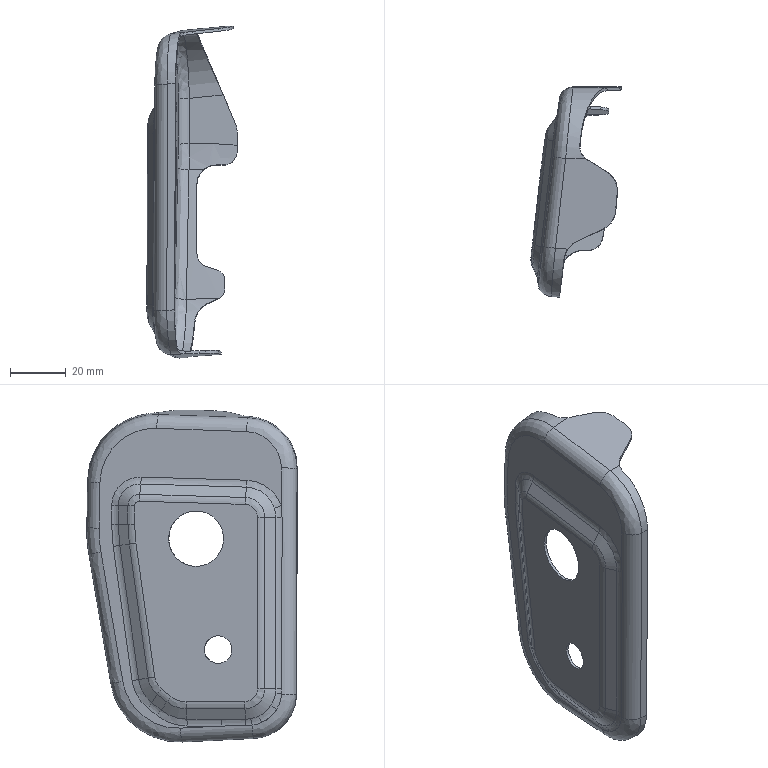Part | 1 solid | 174 faces | box 32.564 x 75.837 x 119.689 mm | volume 10819 mm3 | spline 117 | cylinder 42 | plane 15 | commonest cylinder face diameters 10 x17 8 x10 12 x5 20 x2 30 x1 32 x1